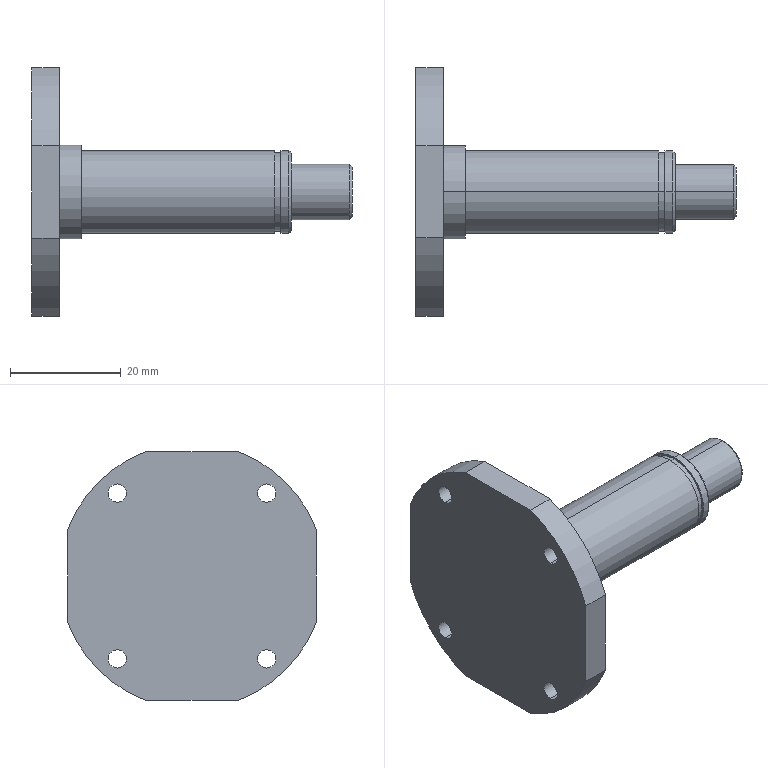Part | SolidWorks | features 3DProfileFeature 1, Chamfer 1, HoleWzd 1, ICE 1, RevCut 1, Revolution 1 | 1 solid | 37 faces | box 58 x 45 x 45 mm | volume 17000 mm3 | cylinder 22 | plane 11 | cone 4 | commonest cylinder face diameters 3.3 x8 15 x4 48 x4 10 x2 14.3 x2 17 x2
STEP:
#1=CARTESIAN_POINT('',(45.1,0.,7.5));
#2=VERTEX_POINT('',#1);
#3=CARTESIAN_POINT('',(45.1,0.,-7.5));
#4=VERTEX_POINT('',#3);
#5=CARTESIAN_POINT('',(45.1,0.,0.));
#6=DIRECTION('',(-1.,0.,0.));
#7=DIRECTION('',(0.,0.,1.));
#8=AXIS2_PLACEMENT_3D('',#5,#6,#7);
#9=CIRCLE('',#8,7.5);
#10=EDGE_CURVE('',#2,#4,#9,.T.);
#11=ORIENTED_EDGE('',*,*,#10,.F.);
#12=CARTESIAN_POINT('',(46.5,0.,7.5));
#13=VERTEX_POINT('',#12);
#14=CARTESIAN_POINT('',(58.,0.,7.5));
#15=DIRECTION('',(1.,0.,0.));
#16=VECTOR('',#15,1000.);
#17=LINE('',#14,#16);
#18=EDGE_CURVE('',#2,#13,#17,.T.);
#19=ORIENTED_EDGE('',*,*,#18,.T.);
#20=CARTESIAN_POINT('',(46.5,0.,-7.5));
#21=VERTEX_POINT('',#20);
#22=CARTESIAN_POINT('',(46.5,0.,0.));
#23=DIRECTION('',(-1.,0.,0.));
#24=DIRECTION('',(0.,0.,-1.));
#25=AXIS2_PLACEMENT_3D('',#22,#23,#24);
#26=CIRCLE('',#25,7.5);
#27=EDGE_CURVE('',#13,#21,#26,.T.);
#28=ORIENTED_EDGE('',*,*,#27,.T.);
#29=CARTESIAN_POINT('',(58.,0.,-7.5));
#30=DIRECTION('',(1.,0.,0.));
#31=VECTOR('',#30,1000.);
#32=LINE('',#29,#31);
#33=EDGE_CURVE('',#4,#21,#32,.T.);
#34=ORIENTED_EDGE('',*,*,#33,.F.);
#35=EDGE_LOOP('',(#11,#19,#28,#34));
#36=FACE_OUTER_BOUND('',#35,.T.);
#37=CARTESIAN_POINT('',(58.,0.,0.));
#38=DIRECTION('',(1.,0.,0.));
#39=DIRECTION('',(0.,0.,-1.));
#40=AXIS2_PLACEMENT_3D('',#37,#38,#39);
#41=CYLINDRICAL_SURFACE('',#40,7.5);
#42=ADVANCED_FACE('',(#36),#41,.T.);
#43=CARTESIAN_POINT('',(47.,0.,-7.));
#44=VERTEX_POINT('',#43);
#45=CARTESIAN_POINT('',(47.,0.,7.));
#46=VERTEX_POINT('',#45);
#47=CARTESIAN_POINT('',(47.,0.,0.));
#48=DIRECTION('',(1.,0.,0.));
#49=DIRECTION('',(0.,0.,-1.));
#50=AXIS2_PLACEMENT_3D('',#47,#48,#49);
#51=CIRCLE('',#50,7.);
#52=EDGE_CURVE('',#44,#46,#51,.T.);
#53=ORIENTED_EDGE('',*,*,#52,.F.);
#54=CARTESIAN_POINT('',(47.,0.,-7.));
#55=DIRECTION('',(-0.7071,0.,-0.7071));
#56=VECTOR('',#55,1000.);
#57=LINE('',#54,#56);
#58=EDGE_CURVE('',#44,#21,#57,.T.);
#59=ORIENTED_EDGE('',*,*,#58,.T.);
#60=ORIENTED_EDGE('',*,*,#27,.F.);
#61=CARTESIAN_POINT('',(47.,0.,7.));
#62=DIRECTION('',(-0.7071,0.,0.7071));
#63=VECTOR('',#62,1000.);
#64=LINE('',#61,#63);
#65=EDGE_CURVE('',#46,#13,#64,.T.);
#66=ORIENTED_EDGE('',*,*,#65,.F.);
#67=EDGE_LOOP('',(#53,#59,#60,#66));
#68=FACE_OUTER_BOUND('',#67,.T.);
#69=CARTESIAN_POINT('',(47.,0.,0.));
#70=DIRECTION('',(-1.,0.,0.));
#71=DIRECTION('',(0.,0.,1.));
#72=AXIS2_PLACEMENT_3D('',#69,#70,#71);
#73=CONICAL_SURFACE('',#72,7.,0.7854);
#74=ADVANCED_FACE('',(#68),#73,.T.);
#75=CARTESIAN_POINT('',(47.,0.,-5.));
#76=VERTEX_POINT('',#75);
#77=CARTESIAN_POINT('',(47.,0.,5.));
#78=VERTEX_POINT('',#77);
#79=CARTESIAN_POINT('',(47.,0.,0.));
#80=DIRECTION('',(1.,0.,0.));
#81=DIRECTION('',(0.,0.,-1.));
#82=AXIS2_PLACEMENT_3D('',#79,#80,#81);
#83=CIRCLE('',#82,5.);
#84=EDGE_CURVE('',#76,#78,#83,.T.);
#85=ORIENTED_EDGE('',*,*,#84,.T.);
#86=CARTESIAN_POINT('',(57.5,0.,5.));
#87=VERTEX_POINT('',#86);
#88=CARTESIAN_POINT('',(58.,0.,5.));
#89=DIRECTION('',(1.,0.,0.));
#90=VECTOR('',#89,1000.);
#91=LINE('',#88,#90);
#92=EDGE_CURVE('',#78,#87,#91,.T.);
#93=ORIENTED_EDGE('',*,*,#92,.T.);
#94=CARTESIAN_POINT('',(57.5,0.,-5.));
#95=VERTEX_POINT('',#94);
#96=CARTESIAN_POINT('',(57.5,0.,0.));
#97=DIRECTION('',(-1.,0.,0.));
#98=DIRECTION('',(0.,0.,-1.));
#99=AXIS2_PLACEMENT_3D('',#96,#97,#98);
#100=CIRCLE('',#99,5.);
#101=EDGE_CURVE('',#87,#95,#100,.T.);
#102=ORIENTED_EDGE('',*,*,#101,.T.);
#103=CARTESIAN_POINT('',(58.,0.,-5.));
#104=DIRECTION('',(1.,0.,0.));
#105=VECTOR('',#104,1000.);
#106=LINE('',#103,#105);
#107=EDGE_CURVE('',#76,#95,#106,.T.);
#108=ORIENTED_EDGE('',*,*,#107,.F.);
#109=EDGE_LOOP('',(#85,#93,#102,#108));
#110=FACE_OUTER_BOUND('',#109,.T.);
#111=CARTESIAN_POINT('',(58.,0.,0.));
#112=DIRECTION('',(1.,0.,0.));
#113=DIRECTION('',(0.,0.,-1.));
#114=AXIS2_PLACEMENT_3D('',#111,#112,#113);
#115=CYLINDRICAL_SURFACE('',#114,5.);
#116=ADVANCED_FACE('',(#110),#115,.T.);
#117=CARTESIAN_POINT('',(58.,0.,-4.5));
#118=VERTEX_POINT('',#117);
#119=CARTESIAN_POINT('',(58.,0.,4.5));
#120=VERTEX_POINT('',#119);
#121=CARTESIAN_POINT('',(58.,0.,0.));
#122=DIRECTION('',(1.,0.,0.));
#123=DIRECTION('',(0.,0.,-1.));
#124=AXIS2_PLACEMENT_3D('',#121,#122,#123);
#125=CIRCLE('',#124,4.5);
#126=EDGE_CURVE('',#118,#120,#125,.T.);
#127=ORIENTED_EDGE('',*,*,#126,.F.);
#128=CARTESIAN_POINT('',(58.,0.,-4.5));
#129=DIRECTION('',(-0.7071,0.,-0.7071));
#130=VECTOR('',#129,1000.);
#131=LINE('',#128,#130);
#132=EDGE_CURVE('',#118,#95,#131,.T.);
#133=ORIENTED_EDGE('',*,*,#132,.T.);
#134=ORIENTED_EDGE('',*,*,#101,.F.);
#135=CARTESIAN_POINT('',(58.,0.,4.5));
#136=DIRECTION('',(-0.7071,0.,0.7071));
#137=VECTOR('',#136,1000.);
#138=LINE('',#135,#137);
#139=EDGE_CURVE('',#120,#87,#138,.T.);
#140=ORIENTED_EDGE('',*,*,#139,.F.);
#141=EDGE_LOOP('',(#127,#133,#134,#140));
#142=FACE_OUTER_BOUND('',#141,.T.);
#143=CARTESIAN_POINT('',(58.,0.,0.));
#144=DIRECTION('',(-1.,0.,0.));
#145=DIRECTION('',(0.,0.,1.));
#146=AXIS2_PLACEMENT_3D('',#143,#144,#145);
#147=CONICAL_SURFACE('',#146,4.5,0.7854);
#148=ADVANCED_FACE('',(#142),#147,.T.);
#149=CARTESIAN_POINT('',(45.1,0.,7.15));
#150=VERTEX_POINT('',#149);
#151=CARTESIAN_POINT('',(45.1,0.,-7.15));
#152=VERTEX_POINT('',#151);
#153=CARTESIAN_POINT('',(45.1,0.,0.));
#154=DIRECTION('',(-1.,0.,0.));
#155=DIRECTION('',(0.,0.,1.));
#156=AXIS2_PLACEMENT_3D('',#153,#154,#155);
#157=CIRCLE('',#156,7.15);
#158=EDGE_CURVE('',#150,#152,#157,.T.);
#159=ORIENTED_EDGE('',*,*,#158,.T.);
#160=CARTESIAN_POINT('',(44.,0.,-7.15));
#161=VERTEX_POINT('',#160);
#162=CARTESIAN_POINT('',(0.,0.,-7.15));
#163=DIRECTION('',(-1.,0.,0.));
#164=VECTOR('',#163,1000.);
#165=LINE('',#162,#164);
#166=EDGE_CURVE('',#152,#161,#165,.T.);
#167=ORIENTED_EDGE('',*,*,#166,.T.);
#168=CARTESIAN_POINT('',(44.,0.,7.15));
#169=VERTEX_POINT('',#168);
#170=CARTESIAN_POINT('',(44.,0.,0.));
#171=DIRECTION('',(-1.,0.,0.));
#172=DIRECTION('',(0.,0.,1.));
#173=AXIS2_PLACEMENT_3D('',#170,#171,#172);
#174=CIRCLE('',#173,7.15);
#175=EDGE_CURVE('',#169,#161,#174,.T.);
#176=ORIENTED_EDGE('',*,*,#175,.F.);
#177=CARTESIAN_POINT('',(0.,0.,7.15));
#178=DIRECTION('',(-1.,0.,0.));
#179=VECTOR('',#178,1000.);
#180=LINE('',#177,#179);
#181=EDGE_CURVE('',#150,#169,#180,.T.);
#182=ORIENTED_EDGE('',*,*,#181,.F.);
#183=EDGE_LOOP('',(#159,#167,#176,#182));
#184=FACE_OUTER_BOUND('',#183,.T.);
#185=CARTESIAN_POINT('',(0.,0.,0.));
#186=DIRECTION('',(-1.,0.,0.));
#187=DIRECTION('',(0.,0.,1.));
#188=AXIS2_PLACEMENT_3D('',#185,#186,#187);
#189=CYLINDRICAL_SURFACE('',#188,7.15);
#190=ADVANCED_FACE('',(#184),#189,.T.);
#191=CARTESIAN_POINT('',(5.,13.5,-13.35));
#192=VERTEX_POINT('',#191);
#193=CARTESIAN_POINT('',(5.,13.5,-16.65));
#194=VERTEX_POINT('',#193);
#195=CARTESIAN_POINT('',(5.,13.5,-15.));
#196=DIRECTION('',(1.,0.,0.));
#197=DIRECTION('',(0.,0.,-1.));
#198=AXIS2_PLACEMENT_3D('',#195,#196,#197);
#199=CIRCLE('',#198,1.65);
#200=EDGE_CURVE('',#192,#194,#199,.T.);
#201=ORIENTED_EDGE('',*,*,#200,.T.);
#202=CARTESIAN_POINT('',(0.,13.5,-16.65));
#203=VERTEX_POINT('',#202);
#204=CARTESIAN_POINT('',(0.,13.5,-16.65));
#205=DIRECTION('',(-1.,0.,0.));
#206=VECTOR('',#205,1000.);
#207=LINE('',#204,#206);
#208=EDGE_CURVE('',#194,#203,#207,.T.);
#209=ORIENTED_EDGE('',*,*,#208,.T.);
#210=CARTESIAN_POINT('',(0.,13.5,-13.35));
#211=VERTEX_POINT('',#210);
#212=CARTESIAN_POINT('',(0.,13.5,-15.));
#213=DIRECTION('',(-1.,0.,0.));
#214=DIRECTION('',(0.,0.,1.));
#215=AXIS2_PLACEMENT_3D('',#212,#213,#214);
#216=CIRCLE('',#215,1.65);
#217=EDGE_CURVE('',#203,#211,#216,.T.);
#218=ORIENTED_EDGE('',*,*,#217,.T.);
#219=CARTESIAN_POINT('',(0.,13.5,-13.35));
#220=DIRECTION('',(-1.,0.,0.));
#221=VECTOR('',#220,1000.);
#222=LINE('',#219,#221);
#223=EDGE_CURVE('',#192,#211,#222,.T.);
#224=ORIENTED_EDGE('',*,*,#223,.F.);
#225=EDGE_LOOP('',(#201,#209,#218,#224));
#226=FACE_OUTER_BOUND('',#225,.T.);
#227=CARTESIAN_POINT('',(0.,13.5,-15.));
#228=DIRECTION('',(-1.,0.,0.));
#229=DIRECTION('',(0.,0.,1.));
#230=AXIS2_PLACEMENT_3D('',#227,#228,#229);
#231=CYLINDRICAL_SURFACE('',#230,1.65);
#232=ADVANCED_FACE('',(#226),#231,.F.);
#233=CARTESIAN_POINT('',(5.,13.5,16.65));
#234=VERTEX_POINT('',#233);
#235=CARTESIAN_POINT('',(5.,13.5,13.35));
#236=VERTEX_POINT('',#235);
#237=CARTESIAN_POINT('',(5.,13.5,15.));
#238=DIRECTION('',(1.,0.,0.));
#239=DIRECTION('',(0.,0.,-1.));
#240=AXIS2_PLACEMENT_3D('',#237,#238,#239);
#241=CIRCLE('',#240,1.65);
#242=EDGE_CURVE('',#234,#236,#241,.T.);
#243=ORIENTED_EDGE('',*,*,#242,.T.);
#244=CARTESIAN_POINT('',(0.,13.5,13.35));
#245=VERTEX_POINT('',#244);
#246=CARTESIAN_POINT('',(0.,13.5,13.35));
#247=DIRECTION('',(-1.,0.,0.));
#248=VECTOR('',#247,1000.);
#249=LINE('',#246,#248);
#250=EDGE_CURVE('',#236,#245,#249,.T.);
#251=ORIENTED_EDGE('',*,*,#250,.T.);
#252=CARTESIAN_POINT('',(0.,13.5,16.65));
#253=VERTEX_POINT('',#252);
#254=CARTESIAN_POINT('',(0.,13.5,15.));
#255=DIRECTION('',(-1.,0.,0.));
#256=DIRECTION('',(0.,0.,1.));
#257=AXIS2_PLACEMENT_3D('',#254,#255,#256);
#258=CIRCLE('',#257,1.65);
#259=EDGE_CURVE('',#245,#253,#258,.T.);
#260=ORIENTED_EDGE('',*,*,#259,.T.);
#261=CARTESIAN_POINT('',(0.,13.5,16.65));
#262=DIRECTION('',(-1.,0.,0.));
#263=VECTOR('',#262,1000.);
#264=LINE('',#261,#263);
#265=EDGE_CURVE('',#234,#253,#264,.T.);
#266=ORIENTED_EDGE('',*,*,#265,.F.);
#267=EDGE_LOOP('',(#243,#251,#260,#266));
#268=FACE_OUTER_BOUND('',#267,.T.);
#269=CARTESIAN_POINT('',(0.,13.5,15.));
#270=DIRECTION('',(-1.,0.,0.));
#271=DIRECTION('',(0.,0.,1.));
#272=AXIS2_PLACEMENT_3D('',#269,#270,#271);
#273=CYLINDRICAL_SURFACE('',#272,1.65);
#274=ADVANCED_FACE('',(#268),#273,.F.);
#275=CARTESIAN_POINT('',(5.,-13.5,-13.35));
#276=VERTEX_POINT('',#275);
#277=CARTESIAN_POINT('',(5.,-13.5,-16.65));
#278=VERTEX_POINT('',#277);
#279=CARTESIAN_POINT('',(5.,-13.5,-15.));
#280=DIRECTION('',(1.,0.,0.));
#281=DIRECTION('',(0.,0.,-1.));
#282=AXIS2_PLACEMENT_3D('',#279,#280,#281);
#283=CIRCLE('',#282,1.65);
#284=EDGE_CURVE('',#276,#278,#283,.T.);
#285=ORIENTED_EDGE('',*,*,#284,.T.);
#286=CARTESIAN_POINT('',(0.,-13.5,-16.65));
#287=VERTEX_POINT('',#286);
#288=CARTESIAN_POINT('',(0.,-13.5,-16.65));
#289=DIRECTION('',(-1.,0.,0.));
#290=VECTOR('',#289,1000.);
#291=LINE('',#288,#290);
#292=EDGE_CURVE('',#278,#287,#291,.T.);
#293=ORIENTED_EDGE('',*,*,#292,.T.);
#294=CARTESIAN_POINT('',(0.,-13.5,-13.35));
#295=VERTEX_POINT('',#294);
#296=CARTESIAN_POINT('',(0.,-13.5,-15.));
#297=DIRECTION('',(-1.,0.,0.));
#298=DIRECTION('',(0.,0.,1.));
#299=AXIS2_PLACEMENT_3D('',#296,#297,#298);
#300=CIRCLE('',#299,1.65);
#301=EDGE_CURVE('',#287,#295,#300,.T.);
#302=ORIENTED_EDGE('',*,*,#301,.T.);
#303=CARTESIAN_POINT('',(0.,-13.5,-13.35));
#304=DIRECTION('',(-1.,0.,0.));
#305=VECTOR('',#304,1000.);
#306=LINE('',#303,#305);
#307=EDGE_CURVE('',#276,#295,#306,.T.);
#308=ORIENTED_EDGE('',*,*,#307,.F.);
#309=EDGE_LOOP('',(#285,#293,#302,#308));
#310=FACE_OUTER_BOUND('',#309,.T.);
#311=CARTESIAN_POINT('',(0.,-13.5,-15.));
#312=DIRECTION('',(-1.,0.,0.));
#313=DIRECTION('',(0.,0.,1.));
#314=AXIS2_PLACEMENT_3D('',#311,#312,#313);
#315=CYLINDRICAL_SURFACE('',#314,1.65);
#316=ADVANCED_FACE('',(#310),#315,.F.);
#317=CARTESIAN_POINT('',(5.,-13.5,16.65));
#318=VERTEX_POINT('',#317);
#319=CARTESIAN_POINT('',(5.,-13.5,13.35));
#320=VERTEX_POINT('',#319);
#321=CARTESIAN_POINT('',(5.,-13.5,15.));
#322=DIRECTION('',(1.,0.,0.));
#323=DIRECTION('',(0.,0.,-1.));
#324=AXIS2_PLACEMENT_3D('',#321,#322,#323);
#325=CIRCLE('',#324,1.65);
#326=EDGE_CURVE('',#318,#320,#325,.T.);
#327=ORIENTED_EDGE('',*,*,#326,.T.);
#328=CARTESIAN_POINT('',(0.,-13.5,13.35));
#329=VERTEX_POINT('',#328);
#330=CARTESIAN_POINT('',(0.,-13.5,13.35));
#331=DIRECTION('',(-1.,0.,0.));
#332=VECTOR('',#331,1000.);
#333=LINE('',#330,#332);
#334=EDGE_CURVE('',#320,#329,#333,.T.);
#335=ORIENTED_EDGE('',*,*,#334,.T.);
#336=CARTESIAN_POINT('',(0.,-13.5,16.65));
#337=VERTEX_POINT('',#336);
#338=CARTESIAN_POINT('',(0.,-13.5,15.));
#339=DIRECTION('',(-1.,0.,0.));
#340=DIRECTION('',(0.,0.,1.));
#341=AXIS2_PLACEMENT_3D('',#338,#339,#340);
#342=CIRCLE('',#341,1.65);
#343=EDGE_CURVE('',#329,#337,#342,.T.);
#344=ORIENTED_EDGE('',*,*,#343,.T.);
#345=CARTESIAN_POINT('',(0.,-13.5,16.65));
#346=DIRECTION('',(-1.,0.,0.));
#347=VECTOR('',#346,1000.);
#348=LINE('',#345,#347);
#349=EDGE_CURVE('',#318,#337,#348,.T.);
#350=ORIENTED_EDGE('',*,*,#349,.F.);
#351=EDGE_LOOP('',(#327,#335,#344,#350));
#352=FACE_OUTER_BOUND('',#351,.T.);
#353=CARTESIAN_POINT('',(0.,-13.5,15.));
#354=DIRECTION('',(-1.,0.,0.));
#355=DIRECTION('',(0.,0.,1.));
#356=AXIS2_PLACEMENT_3D('',#353,#354,#355);
#357=CYLINDRICAL_SURFACE('',#356,1.65);
#358=ADVANCED_FACE('',(#352),#357,.F.);
#359=CARTESIAN_POINT('',(5.,0.,-8.5));
#360=VERTEX_POINT('',#359);
#361=CARTESIAN_POINT('',(5.,0.,8.5));
#362=VERTEX_POINT('',#361);
#363=CARTESIAN_POINT('',(5.,0.,0.));
#364=DIRECTION('',(1.,0.,0.));
#365=DIRECTION('',(0.,0.,-1.));
#366=AXIS2_PLACEMENT_3D('',#363,#364,#365);
#367=CIRCLE('',#366,8.5);
#368=EDGE_CURVE('',#360,#362,#367,.T.);
#369=ORIENTED_EDGE('',*,*,#368,.T.);
#370=CARTESIAN_POINT('',(9.,0.,8.5));
#371=VERTEX_POINT('',#370);
#372=CARTESIAN_POINT('',(58.,0.,8.5));
#373=DIRECTION('',(1.,0.,0.));
#374=VECTOR('',#373,1000.);
#375=LINE('',#372,#374);
#376=EDGE_CURVE('',#362,#371,#375,.T.);
#377=ORIENTED_EDGE('',*,*,#376,.T.);
#378=CARTESIAN_POINT('',(9.,0.,-8.5));
#379=VERTEX_POINT('',#378);
#380=CARTESIAN_POINT('',(9.,0.,0.));
#381=DIRECTION('',(1.,0.,0.));
#382=DIRECTION('',(0.,0.,-1.));
#383=AXIS2_PLACEMENT_3D('',#380,#381,#382);
#384=CIRCLE('',#383,8.5);
#385=EDGE_CURVE('',#379,#371,#384,.T.);
#386=ORIENTED_EDGE('',*,*,#385,.F.);
#387=CARTESIAN_POINT('',(58.,0.,-8.5));
#388=DIRECTION('',(1.,0.,0.));
#389=VECTOR('',#388,1000.);
#390=LINE('',#387,#389);
#391=EDGE_CURVE('',#360,#379,#390,.T.);
#392=ORIENTED_EDGE('',*,*,#391,.F.);
#393=EDGE_LOOP('',(#369,#377,#386,#392));
#394=FACE_OUTER_BOUND('',#393,.T.);
#395=CARTESIAN_POINT('',(58.,0.,0.));
#396=DIRECTION('',(1.,0.,0.));
#397=DIRECTION('',(0.,0.,-1.));
#398=AXIS2_PLACEMENT_3D('',#395,#396,#397);
#399=CYLINDRICAL_SURFACE('',#398,8.5);
#400=ADVANCED_FACE('',(#394),#399,.T.);
#401=CARTESIAN_POINT('',(9.,0.,-7.5));
#402=VERTEX_POINT('',#401);
#403=CARTESIAN_POINT('',(9.,0.,7.5));
#404=VERTEX_POINT('',#403);
#405=CARTESIAN_POINT('',(9.,0.,0.));
#406=DIRECTION('',(1.,0.,0.));
#407=DIRECTION('',(0.,0.,-1.));
#408=AXIS2_PLACEMENT_3D('',#405,#406,#407);
#409=CIRCLE('',#408,7.5);
#410=EDGE_CURVE('',#402,#404,#409,.T.);
#411=ORIENTED_EDGE('',*,*,#410,.T.);
#412=CARTESIAN_POINT('',(44.,0.,7.5));
#413=VERTEX_POINT('',#412);
#414=CARTESIAN_POINT('',(58.,0.,7.5));
#415=DIRECTION('',(1.,0.,0.));
#416=VECTOR('',#415,1000.);
#417=LINE('',#414,#416);
#418=EDGE_CURVE('',#404,#413,#417,.T.);
#419=ORIENTED_EDGE('',*,*,#418,.T.);
#420=CARTESIAN_POINT('',(44.,0.,-7.5));
#421=VERTEX_POINT('',#420);
#422=CARTESIAN_POINT('',(44.,0.,0.));
#423=DIRECTION('',(-1.,0.,0.));
#424=DIRECTION('',(0.,0.,1.));
#425=AXIS2_PLACEMENT_3D('',#422,#423,#424);
#426=CIRCLE('',#425,7.5);
#427=EDGE_CURVE('',#413,#421,#426,.T.);
#428=ORIENTED_EDGE('',*,*,#427,.T.);
#429=CARTESIAN_POINT('',(58.,0.,-7.5));
#430=DIRECTION('',(1.,0.,0.));
#431=VECTOR('',#430,1000.);
#432=LINE('',#429,#431);
#433=EDGE_CURVE('',#402,#421,#432,.T.);
#434=ORIENTED_EDGE('',*,*,#433,.F.);
#435=EDGE_LOOP('',(#411,#419,#428,#434));
#436=FACE_OUTER_BOUND('',#435,.T.);
#437=CARTESIAN_POINT('',(58.,0.,0.));
#438=DIRECTION('',(1.,0.,0.));
#439=DIRECTION('',(0.,0.,-1.));
#440=AXIS2_PLACEMENT_3D('',#437,#438,#439);
#441=CYLINDRICAL_SURFACE('',#440,7.5);
#442=ADVANCED_FACE('',(#436),#441,.T.);
#443=ORIENTED_EDGE('',*,*,#418,.F.);
#444=CARTESIAN_POINT('',(9.,0.,0.));
#445=DIRECTION('',(1.,0.,0.));
#446=DIRECTION('',(0.,0.,-1.));
#447=AXIS2_PLACEMENT_3D('',#444,#445,#446);
#448=CIRCLE('',#447,7.5);
#449=EDGE_CURVE('',#404,#402,#448,.T.);
#450=ORIENTED_EDGE('',*,*,#449,.T.);
#451=ORIENTED_EDGE('',*,*,#433,.T.);
#452=CARTESIAN_POINT('',(44.,0.,0.));
#453=DIRECTION('',(-1.,0.,0.));
#454=DIRECTION('',(0.,0.,1.));
#455=AXIS2_PLACEMENT_3D('',#452,#453,#454);
#456=CIRCLE('',#455,7.5);
#457=EDGE_CURVE('',#421,#413,#456,.T.);
#458=ORIENTED_EDGE('',*,*,#457,.T.);
#459=EDGE_LOOP('',(#443,#450,#451,#458));
#460=FACE_OUTER_BOUND('',#459,.T.);
#461=CARTESIAN_POINT('',(58.,0.,0.));
#462=DIRECTION('',(1.,0.,0.));
#463=DIRECTION('',(0.,0.,-1.));
#464=AXIS2_PLACEMENT_3D('',#461,#462,#463);
#465=CYLINDRICAL_SURFACE('',#464,7.5);
#466=ADVANCED_FACE('',(#460),#465,.T.);
#467=CARTESIAN_POINT('',(0.,13.5,-15.));
#468=DIRECTION('',(-1.,0.,0.));
#469=DIRECTION('',(0.,0.,1.));
#470=AXIS2_PLACEMENT_3D('',#467,#468,#469);
#471=CIRCLE('',#470,1.65);
#472=EDGE_CURVE('',#211,#203,#471,.T.);
#473=ORIENTED_EDGE('',*,*,#472,.F.);
#474=ORIENTED_EDGE('',*,*,#217,.F.);
#475=EDGE_LOOP('',(#473,#474));
#476=FACE_BOUND('',#475,.T.);
#477=CARTESIAN_POINT('',(0.,13.5,15.));
#478=DIRECTION('',(-1.,0.,0.));
#479=DIRECTION('',(0.,0.,1.));
#480=AXIS2_PLACEMENT_3D('',#477,#478,#479);
#481=CIRCLE('',#480,1.65);
#482=EDGE_CURVE('',#253,#245,#481,.T.);
#483=ORIENTED_EDGE('',*,*,#482,.F.);
#484=ORIENTED_EDGE('',*,*,#259,.F.);
#485=EDGE_LOOP('',(#483,#484));
#486=FACE_BOUND('',#485,.T.);
#487=CARTESIAN_POINT('',(0.,-13.5,-15.));
#488=DIRECTION('',(-1.,0.,0.));
#489=DIRECTION('',(0.,0.,1.));
#490=AXIS2_PLACEMENT_3D('',#487,#488,#489);
#491=CIRCLE('',#490,1.65);
#492=EDGE_CURVE('',#295,#287,#491,.T.);
#493=ORIENTED_EDGE('',*,*,#492,.F.);
#494=ORIENTED_EDGE('',*,*,#301,.F.);
#495=EDGE_LOOP('',(#493,#494));
#496=FACE_BOUND('',#495,.T.);
#497=CARTESIAN_POINT('',(0.,-13.5,15.));
#498=DIRECTION('',(-1.,0.,0.));
#499=DIRECTION('',(0.,0.,1.));
#500=AXIS2_PLACEMENT_3D('',#497,#498,#499);
#501=CIRCLE('',#500,1.65);
#502=EDGE_CURVE('',#337,#329,#501,.T.);
#503=ORIENTED_EDGE('',*,*,#502,.F.);
#504=ORIENTED_EDGE('',*,*,#343,.F.);
#505=EDGE_LOOP('',(#503,#504));
#506=FACE_BOUND('',#505,.T.);
#507=CARTESIAN_POINT('',(0.,-8.352,22.5));
#508=VERTEX_POINT('',#507);
#509=CARTESIAN_POINT('',(0.,-22.5,8.352));
#510=VERTEX_POINT('',#509);
#511=CARTESIAN_POINT('',(0.,0.,0.));
#512=DIRECTION('',(1.,0.,0.));
#513=DIRECTION('',(0.,0.,-1.));
#514=AXIS2_PLACEMENT_3D('',#511,#512,#513);
#515=CIRCLE('',#514,24.);
#516=EDGE_CURVE('',#508,#510,#515,.T.);
#517=ORIENTED_EDGE('',*,*,#516,.F.);
#518=CARTESIAN_POINT('',(0.,8.352,22.5));
#519=VERTEX_POINT('',#518);
#520=CARTESIAN_POINT('',(0.,-22.5,22.5));
#521=DIRECTION('',(0.,1.,0.));
#522=VECTOR('',#521,1000.);
#523=LINE('',#520,#522);
#524=EDGE_CURVE('',#508,#519,#523,.T.);
#525=ORIENTED_EDGE('',*,*,#524,.T.);
#526=CARTESIAN_POINT('',(0.,22.5,8.352));
#527=VERTEX_POINT('',#526);
#528=CARTESIAN_POINT('',(0.,0.,0.));
#529=DIRECTION('',(1.,0.,0.));
#530=DIRECTION('',(0.,0.,-1.));
#531=AXIS2_PLACEMENT_3D('',#528,#529,#530);
#532=CIRCLE('',#531,24.);
#533=EDGE_CURVE('',#527,#519,#532,.T.);
#534=ORIENTED_EDGE('',*,*,#533,.F.);
#535=CARTESIAN_POINT('',(0.,22.5,-8.352));
#536=VERTEX_POINT('',#535);
#537=CARTESIAN_POINT('',(0.,22.5,-22.5));
#538=DIRECTION('',(0.,0.,-1.));
#539=VECTOR('',#538,1000.);
#540=LINE('',#537,#539);
#541=EDGE_CURVE('',#527,#536,#540,.T.);
#542=ORIENTED_EDGE('',*,*,#541,.T.);
#543=CARTESIAN_POINT('',(0.,8.352,-22.5));
#544=VERTEX_POINT('',#543);
#545=CARTESIAN_POINT('',(0.,0.,0.));
#546=DIRECTION('',(1.,0.,0.));
#547=DIRECTION('',(0.,0.,-1.));
#548=AXIS2_PLACEMENT_3D('',#545,#546,#547);
#549=CIRCLE('',#548,24.);
#550=EDGE_CURVE('',#544,#536,#549,.T.);
#551=ORIENTED_EDGE('',*,*,#550,.F.);
#552=CARTESIAN_POINT('',(0.,-8.352,-22.5));
#553=VERTEX_POINT('',#552);
#554=CARTESIAN_POINT('',(0.,-22.5,-22.5));
#555=DIRECTION('',(0.,-1.,0.));
#556=VECTOR('',#555,1000.);
#557=LINE('',#554,#556);
#558=EDGE_CURVE('',#544,#553,#557,.T.);
#559=ORIENTED_EDGE('',*,*,#558,.T.);
#560=CARTESIAN_POINT('',(0.,-22.5,-8.352));
#561=VERTEX_POINT('',#560);
#562=CARTESIAN_POINT('',(0.,0.,0.));
#563=DIRECTION('',(1.,0.,0.));
#564=DIRECTION('',(0.,0.,-1.));
#565=AXIS2_PLACEMENT_3D('',#562,#563,#564);
#566=CIRCLE('',#565,24.);
#567=EDGE_CURVE('',#561,#553,#566,.T.);
#568=ORIENTED_EDGE('',*,*,#567,.F.);
#569=CARTESIAN_POINT('',(0.,-22.5,-22.5));
#570=DIRECTION('',(0.,0.,1.));
#571=VECTOR('',#570,1000.);
#572=LINE('',#569,#571);
#573=EDGE_CURVE('',#561,#510,#572,.T.);
#574=ORIENTED_EDGE('',*,*,#573,.T.);
#575=EDGE_LOOP('',(#517,#525,#534,#542,#551,#559,#568,#574));
#576=FACE_OUTER_BOUND('',#575,.T.);
#577=CARTESIAN_POINT('',(0.,0.,0.));
#578=DIRECTION('',(-1.,0.,0.));
#579=DIRECTION('',(0.,0.,1.));
#580=AXIS2_PLACEMENT_3D('',#577,#578,#579);
#581=PLANE('',#580);
#582=ADVANCED_FACE('',(#476,#486,#496,#506,#576),#581,.T.);
#583=CARTESIAN_POINT('',(5.,-8.352,22.5));
#584=VERTEX_POINT('',#583);
#585=CARTESIAN_POINT('',(5.,-22.5,8.352));
#586=VERTEX_POINT('',#585);
#587=CARTESIAN_POINT('',(5.,0.,0.));
#588=DIRECTION('',(1.,0.,0.));
#589=DIRECTION('',(0.,0.,-1.));
#590=AXIS2_PLACEMENT_3D('',#587,#588,#589);
#591=CIRCLE('',#590,24.);
#592=EDGE_CURVE('',#584,#586,#591,.T.);
#593=ORIENTED_EDGE('',*,*,#592,.F.);
#594=CARTESIAN_POINT('',(58.,-8.352,22.5));
#595=DIRECTION('',(-1.,0.,0.));
#596=VECTOR('',#595,1000.);
#597=LINE('',#594,#596);
#598=EDGE_CURVE('',#584,#508,#597,.T.);
#599=ORIENTED_EDGE('',*,*,#598,.T.);
#600=ORIENTED_EDGE('',*,*,#516,.T.);
#601=CARTESIAN_POINT('',(58.,-22.5,8.352));
#602=DIRECTION('',(1.,0.,0.));
#603=VECTOR('',#602,1000.);
#604=LINE('',#601,#603);
#605=EDGE_CURVE('',#510,#586,#604,.T.);
#606=ORIENTED_EDGE('',*,*,#605,.T.);
#607=EDGE_LOOP('',(#593,#599,#600,#606));
#608=FACE_OUTER_BOUND('',#607,.T.);
#609=CARTESIAN_POINT('',(58.,0.,0.));
#610=DIRECTION('',(1.,0.,0.));
#611=DIRECTION('',(0.,0.,-1.));
#612=AXIS2_PLACEMENT_3D('',#609,#610,#611);
#613=CYLINDRICAL_SURFACE('',#612,24.);
#614=ADVANCED_FACE('',(#608),#613,.T.);
#615=ORIENTED_EDGE('',*,*,#533,.T.);
#616=CARTESIAN_POINT('',(5.,8.352,22.5));
#617=VERTEX_POINT('',#616);
#618=CARTESIAN_POINT('',(58.,8.352,22.5));
#619=DIRECTION('',(1.,0.,0.));
#620=VECTOR('',#619,1000.);
#621=LINE('',#618,#620);
#622=EDGE_CURVE('',#519,#617,#621,.T.);
#623=ORIENTED_EDGE('',*,*,#622,.T.);
#624=CARTESIAN_POINT('',(5.,22.5,8.352));
#625=VERTEX_POINT('',#624);
#626=CARTESIAN_POINT('',(5.,0.,0.));
#627=DIRECTION('',(1.,0.,0.));
#628=DIRECTION('',(0.,0.,-1.));
#629=AXIS2_PLACEMENT_3D('',#626,#627,#628);
#630=CIRCLE('',#629,24.);
#631=EDGE_CURVE('',#625,#617,#630,.T.);
#632=ORIENTED_EDGE('',*,*,#631,.F.);
#633=CARTESIAN_POINT('',(58.,22.5,8.352));
#634=DIRECTION('',(-1.,0.,0.));
#635=VECTOR('',#634,1000.);
#636=LINE('',#633,#635);
#637=EDGE_CURVE('',#625,#527,#636,.T.);
#638=ORIENTED_EDGE('',*,*,#637,.T.);
#639=EDGE_LOOP('',(#615,#623,#632,#638));
#640=FACE_OUTER_BOUND('',#639,.T.);
#641=CARTESIAN_POINT('',(58.,0.,0.));
#642=DIRECTION('',(1.,0.,0.));
#643=DIRECTION('',(0.,0.,-1.));
#644=AXIS2_PLACEMENT_3D('',#641,#642,#643);
#645=CYLINDRICAL_SURFACE('',#644,24.);
#646=ADVANCED_FACE('',(#640),#645,.T.);
#647=CARTESIAN_POINT('',(5.,-22.5,-8.352));
#648=VERTEX_POINT('',#647);
#649=CARTESIAN_POINT('',(5.,-8.352,-22.5));
#650=VERTEX_POINT('',#649);
#651=CARTESIAN_POINT('',(5.,0.,0.));
#652=DIRECTION('',(1.,0.,0.));
#653=DIRECTION('',(0.,0.,-1.));
#654=AXIS2_PLACEMENT_3D('',#651,#652,#653);
#655=CIRCLE('',#654,24.);
#656=EDGE_CURVE('',#648,#650,#655,.T.);
#657=ORIENTED_EDGE('',*,*,#656,.F.);
#658=CARTESIAN_POINT('',(58.,-22.5,-8.352));
#659=DIRECTION('',(-1.,0.,0.));
#660=VECTOR('',#659,1000.);
#661=LINE('',#658,#660);
#662=EDGE_CURVE('',#648,#561,#661,.T.);
#663=ORIENTED_EDGE('',*,*,#662,.T.);
#664=ORIENTED_EDGE('',*,*,#567,.T.);
#665=CARTESIAN_POINT('',(58.,-8.352,-22.5));
#666=DIRECTION('',(1.,0.,0.));
#667=VECTOR('',#666,1000.);
#668=LINE('',#665,#667);
#669=EDGE_CURVE('',#553,#650,#668,.T.);
#670=ORIENTED_EDGE('',*,*,#669,.T.);
#671=EDGE_LOOP('',(#657,#663,#664,#670));
#672=FACE_OUTER_BOUND('',#671,.T.);
#673=CARTESIAN_POINT('',(58.,0.,0.));
#674=DIRECTION('',(1.,0.,0.));
#675=DIRECTION('',(0.,0.,-1.));
#676=AXIS2_PLACEMENT_3D('',#673,#674,#675);
#677=CYLINDRICAL_SURFACE('',#676,24.);
#678=ADVANCED_FACE('',(#672),#677,.T.);
#679=CARTESIAN_POINT('',(5.,8.352,-22.5));
#680=VERTEX_POINT('',#679);
#681=CARTESIAN_POINT('',(5.,22.5,-8.352));
#682=VERTEX_POINT('',#681);
#683=CARTESIAN_POINT('',(5.,0.,0.));
#684=DIRECTION('',(1.,0.,0.));
#685=DIRECTION('',(0.,0.,-1.));
#686=AXIS2_PLACEMENT_3D('',#683,#684,#685);
#687=CIRCLE('',#686,24.);
#688=EDGE_CURVE('',#680,#682,#687,.T.);
#689=ORIENTED_EDGE('',*,*,#688,.F.);
#690=CARTESIAN_POINT('',(58.,8.352,-22.5));
#691=DIRECTION('',(-1.,0.,0.));
#692=VECTOR('',#691,1000.);
#693=LINE('',#690,#692);
#694=EDGE_CURVE('',#680,#544,#693,.T.);
#695=ORIENTED_EDGE('',*,*,#694,.T.);
#696=ORIENTED_EDGE('',*,*,#550,.T.);
#697=CARTESIAN_POINT('',(58.,22.5,-8.352));
#698=DIRECTION('',(1.,0.,0.));
#699=VECTOR('',#698,1000.);
#700=LINE('',#697,#699);
#701=EDGE_CURVE('',#536,#682,#700,.T.);
#702=ORIENTED_EDGE('',*,*,#701,.T.);
#703=EDGE_LOOP('',(#689,#695,#696,#702));
#704=FACE_OUTER_BOUND('',#703,.T.);
#705=CARTESIAN_POINT('',(58.,0.,0.));
#706=DIRECTION('',(1.,0.,0.));
#707=DIRECTION('',(0.,0.,-1.));
#708=AXIS2_PLACEMENT_3D('',#705,#706,#707);
#709=CYLINDRICAL_SURFACE('',#708,24.);
#710=ADVANCED_FACE('',(#704),#709,.T.);
#711=ORIENTED_EDGE('',*,*,#200,.F.);
#712=CARTESIAN_POINT('',(5.,13.5,-15.));
#713=DIRECTION('',(1.,0.,0.));
#714=DIRECTION('',(0.,0.,-1.));
#715=AXIS2_PLACEMENT_3D('',#712,#713,#714);
#716=CIRCLE('',#715,1.65);
#717=EDGE_CURVE('',#194,#192,#716,.T.);
#718=ORIENTED_EDGE('',*,*,#717,.F.);
#719=EDGE_LOOP('',(#711,#718));
#720=FACE_BOUND('',#719,.T.);
#721=ORIENTED_EDGE('',*,*,#242,.F.);
#722=CARTESIAN_POINT('',(5.,13.5,15.));
#723=DIRECTION('',(1.,0.,0.));
#724=DIRECTION('',(0.,0.,-1.));
#725=AXIS2_PLACEMENT_3D('',#722,#723,#724);
#726=CIRCLE('',#725,1.65);
#727=EDGE_CURVE('',#236,#234,#726,.T.);
#728=ORIENTED_EDGE('',*,*,#727,.F.);
#729=EDGE_LOOP('',(#721,#728));
#730=FACE_BOUND('',#729,.T.);
#731=ORIENTED_EDGE('',*,*,#284,.F.);
#732=CARTESIAN_POINT('',(5.,-13.5,-15.));
#733=DIRECTION('',(1.,0.,0.));
#734=DIRECTION('',(0.,0.,-1.));
#735=AXIS2_PLACEMENT_3D('',#732,#733,#734);
#736=CIRCLE('',#735,1.65);
#737=EDGE_CURVE('',#278,#276,#736,.T.);
#738=ORIENTED_EDGE('',*,*,#737,.F.);
#739=EDGE_LOOP('',(#731,#738));
#740=FACE_BOUND('',#739,.T.);
#741=ORIENTED_EDGE('',*,*,#326,.F.);
#742=CARTESIAN_POINT('',(5.,-13.5,15.));
#743=DIRECTION('',(1.,0.,0.));
#744=DIRECTION('',(0.,0.,-1.));
#745=AXIS2_PLACEMENT_3D('',#742,#743,#744);
#746=CIRCLE('',#745,1.65);
#747=EDGE_CURVE('',#320,#318,#746,.T.);
#748=ORIENTED_EDGE('',*,*,#747,.F.);
#749=EDGE_LOOP('',(#741,#748));
#750=FACE_BOUND('',#749,.T.);
#751=ORIENTED_EDGE('',*,*,#368,.F.);
#752=CARTESIAN_POINT('',(5.,0.,0.));
#753=DIRECTION('',(1.,0.,0.));
#754=DIRECTION('',(0.,0.,-1.));
#755=AXIS2_PLACEMENT_3D('',#752,#753,#754);
#756=CIRCLE('',#755,8.5);
#757=EDGE_CURVE('',#362,#360,#756,.T.);
#758=ORIENTED_EDGE('',*,*,#757,.F.);
#759=EDGE_LOOP('',(#751,#758));
#760=FACE_BOUND('',#759,.T.);
#761=ORIENTED_EDGE('',*,*,#631,.T.);
#762=CARTESIAN_POINT('',(5.,0.,22.5));
#763=DIRECTION('',(0.,-1.,0.));
#764=VECTOR('',#763,1000.);
#765=LINE('',#762,#764);
#766=EDGE_CURVE('',#617,#584,#765,.T.);
#767=ORIENTED_EDGE('',*,*,#766,.T.);
#768=ORIENTED_EDGE('',*,*,#592,.T.);
#769=CARTESIAN_POINT('',(5.,-22.5,-24.));
#770=DIRECTION('',(0.,0.,-1.));
#771=VECTOR('',#770,1000.);
#772=LINE('',#769,#771);
#773=EDGE_CURVE('',#586,#648,#772,.T.);
#774=ORIENTED_EDGE('',*,*,#773,.T.);
#775=ORIENTED_EDGE('',*,*,#656,.T.);
#776=CARTESIAN_POINT('',(5.,0.,-22.5));
#777=DIRECTION('',(0.,1.,0.));
#778=VECTOR('',#777,1000.);
#779=LINE('',#776,#778);
#780=EDGE_CURVE('',#650,#680,#779,.T.);
#781=ORIENTED_EDGE('',*,*,#780,.T.);
#782=ORIENTED_EDGE('',*,*,#688,.T.);
#783=CARTESIAN_POINT('',(5.,22.5,-24.));
#784=DIRECTION('',(0.,0.,1.));
#785=VECTOR('',#784,1000.);
#786=LINE('',#783,#785);
#787=EDGE_CURVE('',#682,#625,#786,.T.);
#788=ORIENTED_EDGE('',*,*,#787,.T.);
#789=EDGE_LOOP('',(#761,#767,#768,#774,#775,#781,#782,#788));
#790=FACE_OUTER_BOUND('',#789,.T.);
#791=CARTESIAN_POINT('',(5.,0.,-24.));
#792=DIRECTION('',(1.,0.,0.));
#793=DIRECTION('',(0.,0.,-1.));
#794=AXIS2_PLACEMENT_3D('',#791,#792,#793);
#795=PLANE('',#794);
#796=ADVANCED_FACE('',(#720,#730,#740,#750,#760,#790),#795,.T.);
#797=ORIENTED_EDGE('',*,*,#376,.F.);
#798=ORIENTED_EDGE('',*,*,#757,.T.);
#799=ORIENTED_EDGE('',*,*,#391,.T.);
#800=CARTESIAN_POINT('',(9.,0.,0.));
#801=DIRECTION('',(1.,0.,0.));
#802=DIRECTION('',(0.,0.,-1.));
#803=AXIS2_PLACEMENT_3D('',#800,#801,#802);
#804=CIRCLE('',#803,8.5);
#805=EDGE_CURVE('',#371,#379,#804,.T.);
#806=ORIENTED_EDGE('',*,*,#805,.F.);
#807=EDGE_LOOP('',(#797,#798,#799,#806));
#808=FACE_OUTER_BOUND('',#807,.T.);
#809=CARTESIAN_POINT('',(58.,0.,0.));
#810=DIRECTION('',(1.,0.,0.));
#811=DIRECTION('',(0.,0.,-1.));
#812=AXIS2_PLACEMENT_3D('',#809,#810,#811);
#813=CYLINDRICAL_SURFACE('',#812,8.5);
#814=ADVANCED_FACE('',(#808),#813,.T.);
#815=ORIENTED_EDGE('',*,*,#385,.T.);
#816=ORIENTED_EDGE('',*,*,#805,.T.);
#817=EDGE_LOOP('',(#815,#816));
#818=FACE_OUTER_BOUND('',#817,.T.);
#819=ORIENTED_EDGE('',*,*,#410,.F.);
#820=ORIENTED_EDGE('',*,*,#449,.F.);
#821=EDGE_LOOP('',(#819,#820));
#822=FACE_BOUND('',#821,.T.);
#823=CARTESIAN_POINT('',(9.,0.,-8.5));
#824=DIRECTION('',(1.,0.,0.));
#825=DIRECTION('',(0.,0.,-1.));
#826=AXIS2_PLACEMENT_3D('',#823,#824,#825);
#827=PLANE('',#826);
#828=ADVANCED_FACE('',(#818,#822),#827,.T.);
#829=ORIENTED_EDGE('',*,*,#334,.F.);
#830=ORIENTED_EDGE('',*,*,#747,.T.);
#831=ORIENTED_EDGE('',*,*,#349,.T.);
#832=ORIENTED_EDGE('',*,*,#502,.T.);
#833=EDGE_LOOP('',(#829,#830,#831,#832));
#834=FACE_OUTER_BOUND('',#833,.T.);
#835=CARTESIAN_POINT('',(0.,-13.5,15.));
#836=DIRECTION('',(-1.,0.,0.));
#837=DIRECTION('',(0.,0.,1.));
#838=AXIS2_PLACEMENT_3D('',#835,#836,#837);
#839=CYLINDRICAL_SURFACE('',#838,1.65);
#840=ADVANCED_FACE('',(#834),#839,.F.);
#841=ORIENTED_EDGE('',*,*,#292,.F.);
#842=ORIENTED_EDGE('',*,*,#737,.T.);
#843=ORIENTED_EDGE('',*,*,#307,.T.);
#844=ORIENTED_EDGE('',*,*,#492,.T.);
#845=EDGE_LOOP('',(#841,#842,#843,#844));
#846=FACE_OUTER_BOUND('',#845,.T.);
#847=CARTESIAN_POINT('',(0.,-13.5,-15.));
#848=DIRECTION('',(-1.,0.,0.));
#849=DIRECTION('',(0.,0.,1.));
#850=AXIS2_PLACEMENT_3D('',#847,#848,#849);
#851=CYLINDRICAL_SURFACE('',#850,1.65);
#852=ADVANCED_FACE('',(#846),#851,.F.);
#853=ORIENTED_EDGE('',*,*,#250,.F.);
#854=ORIENTED_EDGE('',*,*,#727,.T.);
#855=ORIENTED_EDGE('',*,*,#265,.T.);
#856=ORIENTED_EDGE('',*,*,#482,.T.);
#857=EDGE_LOOP('',(#853,#854,#855,#856));
#858=FACE_OUTER_BOUND('',#857,.T.);
#859=CARTESIAN_POINT('',(0.,13.5,15.));
#860=DIRECTION('',(-1.,0.,0.));
#861=DIRECTION('',(0.,0.,1.));
#862=AXIS2_PLACEMENT_3D('',#859,#860,#861);
#863=CYLINDRICAL_SURFACE('',#862,1.65);
#864=ADVANCED_FACE('',(#858),#863,.F.);
#865=ORIENTED_EDGE('',*,*,#208,.F.);
#866=ORIENTED_EDGE('',*,*,#717,.T.);
#867=ORIENTED_EDGE('',*,*,#223,.T.);
#868=ORIENTED_EDGE('',*,*,#472,.T.);
#869=EDGE_LOOP('',(#865,#866,#867,#868));
#870=FACE_OUTER_BOUND('',#869,.T.);
#871=CARTESIAN_POINT('',(0.,13.5,-15.));
#872=DIRECTION('',(-1.,0.,0.));
#873=DIRECTION('',(0.,0.,1.));
#874=AXIS2_PLACEMENT_3D('',#871,#872,#873);
#875=CYLINDRICAL_SURFACE('',#874,1.65);
#876=ADVANCED_FACE('',(#870),#875,.F.);
#877=ORIENTED_EDGE('',*,*,#787,.F.);
#878=ORIENTED_EDGE('',*,*,#701,.F.);
#879=ORIENTED_EDGE('',*,*,#541,.F.);
#880=ORIENTED_EDGE('',*,*,#637,.F.);
#881=EDGE_LOOP('',(#877,#878,#879,#880));
#882=FACE_OUTER_BOUND('',#881,.T.);
#883=CARTESIAN_POINT('',(10.,22.5,-22.5));
#884=DIRECTION('',(0.,1.,0.));
#885=DIRECTION('',(0.,0.,1.));
#886=AXIS2_PLACEMENT_3D('',#883,#884,#885);
#887=PLANE('',#886);
#888=ADVANCED_FACE('',(#882),#887,.T.);
#889=ORIENTED_EDGE('',*,*,#780,.F.);
#890=ORIENTED_EDGE('',*,*,#669,.F.);
#891=ORIENTED_EDGE('',*,*,#558,.F.);
#892=ORIENTED_EDGE('',*,*,#694,.F.);
#893=EDGE_LOOP('',(#889,#890,#891,#892));
#894=FACE_OUTER_BOUND('',#893,.T.);
#895=CARTESIAN_POINT('',(10.,-22.5,-22.5));
#896=DIRECTION('',(0.,0.,-1.));
#897=DIRECTION('',(-1.,0.,0.));
#898=AXIS2_PLACEMENT_3D('',#895,#896,#897);
#899=PLANE('',#898);
#900=ADVANCED_FACE('',(#894),#899,.T.);
#901=ORIENTED_EDGE('',*,*,#773,.F.);
#902=ORIENTED_EDGE('',*,*,#605,.F.);
#903=ORIENTED_EDGE('',*,*,#573,.F.);
#904=ORIENTED_EDGE('',*,*,#662,.F.);
#905=EDGE_LOOP('',(#901,#902,#903,#904));
#906=FACE_OUTER_BOUND('',#905,.T.);
#907=CARTESIAN_POINT('',(10.,-22.5,-22.5));
#908=DIRECTION('',(0.,-1.,0.));
#909=DIRECTION('',(0.,0.,-1.));
#910=AXIS2_PLACEMENT_3D('',#907,#908,#909);
#911=PLANE('',#910);
#912=ADVANCED_FACE('',(#906),#911,.T.);
#913=ORIENTED_EDGE('',*,*,#766,.F.);
#914=ORIENTED_EDGE('',*,*,#622,.F.);
#915=ORIENTED_EDGE('',*,*,#524,.F.);
#916=ORIENTED_EDGE('',*,*,#598,.F.);
#917=EDGE_LOOP('',(#913,#914,#915,#916));
#918=FACE_OUTER_BOUND('',#917,.T.);
#919=CARTESIAN_POINT('',(10.,-22.5,22.5));
#920=DIRECTION('',(0.,0.,1.));
#921=DIRECTION('',(1.,0.,0.));
#922=AXIS2_PLACEMENT_3D('',#919,#920,#921);
#923=PLANE('',#922);
#924=ADVANCED_FACE('',(#918),#923,.T.);
#925=ORIENTED_EDGE('',*,*,#175,.T.);
#926=CARTESIAN_POINT('',(44.,0.,0.));
#927=DIRECTION('',(-1.,0.,0.));
#928=DIRECTION('',(0.,0.,1.));
#929=AXIS2_PLACEMENT_3D('',#926,#927,#928);
#930=CIRCLE('',#929,7.15);
#931=EDGE_CURVE('',#161,#169,#930,.T.);
#932=ORIENTED_EDGE('',*,*,#931,.T.);
#933=EDGE_LOOP('',(#925,#932));
#934=FACE_BOUND('',#933,.T.);
#935=ORIENTED_EDGE('',*,*,#457,.F.);
#936=ORIENTED_EDGE('',*,*,#427,.F.);
#937=EDGE_LOOP('',(#935,#936));
#938=FACE_OUTER_BOUND('',#937,.T.);
#939=CARTESIAN_POINT('',(44.,0.,-7.5));
#940=DIRECTION('',(1.,0.,0.));
#941=DIRECTION('',(0.,0.,-1.));
#942=AXIS2_PLACEMENT_3D('',#939,#940,#941);
#943=PLANE('',#942);
#944=ADVANCED_FACE('',(#934,#938),#943,.T.);
#945=ORIENTED_EDGE('',*,*,#166,.F.);
#946=CARTESIAN_POINT('',(45.1,0.,0.));
#947=DIRECTION('',(-1.,0.,0.));
#948=DIRECTION('',(0.,0.,1.));
#949=AXIS2_PLACEMENT_3D('',#946,#947,#948);
#950=CIRCLE('',#949,7.15);
#951=EDGE_CURVE('',#152,#150,#950,.T.);
#952=ORIENTED_EDGE('',*,*,#951,.T.);
#953=ORIENTED_EDGE('',*,*,#181,.T.);
#954=ORIENTED_EDGE('',*,*,#931,.F.);
#955=EDGE_LOOP('',(#945,#952,#953,#954));
#956=FACE_OUTER_BOUND('',#955,.T.);
#957=CARTESIAN_POINT('',(0.,0.,0.));
#958=DIRECTION('',(-1.,0.,0.));
#959=DIRECTION('',(0.,0.,1.));
#960=AXIS2_PLACEMENT_3D('',#957,#958,#959);
#961=CYLINDRICAL_SURFACE('',#960,7.15);
#962=ADVANCED_FACE('',(#956),#961,.T.);
#963=CARTESIAN_POINT('',(45.1,0.,0.));
#964=DIRECTION('',(-1.,0.,0.));
#965=DIRECTION('',(0.,0.,1.));
#966=AXIS2_PLACEMENT_3D('',#963,#964,#965);
#967=CIRCLE('',#966,7.5);
#968=EDGE_CURVE('',#4,#2,#967,.T.);
#969=ORIENTED_EDGE('',*,*,#968,.T.);
#970=ORIENTED_EDGE('',*,*,#10,.T.);
#971=EDGE_LOOP('',(#969,#970));
#972=FACE_OUTER_BOUND('',#971,.T.);
#973=ORIENTED_EDGE('',*,*,#158,.F.);
#974=ORIENTED_EDGE('',*,*,#951,.F.);
#975=EDGE_LOOP('',(#973,#974));
#976=FACE_BOUND('',#975,.T.);
#977=CARTESIAN_POINT('',(45.1,0.,-7.5));
#978=DIRECTION('',(-1.,0.,0.));
#979=DIRECTION('',(0.,0.,1.));
#980=AXIS2_PLACEMENT_3D('',#977,#978,#979);
#981=PLANE('',#980);
#982=ADVANCED_FACE('',(#972,#976),#981,.T.);
#983=CARTESIAN_POINT('',(58.,0.,0.));
#984=DIRECTION('',(1.,0.,0.));
#985=DIRECTION('',(0.,0.,-1.));
#986=AXIS2_PLACEMENT_3D('',#983,#984,#985);
#987=CIRCLE('',#986,4.5);
#988=EDGE_CURVE('',#120,#118,#987,.T.);
#989=ORIENTED_EDGE('',*,*,#988,.T.);
#990=ORIENTED_EDGE('',*,*,#126,.T.);
#991=EDGE_LOOP('',(#989,#990));
#992=FACE_OUTER_BOUND('',#991,.T.);
#993=CARTESIAN_POINT('',(58.,0.,-5.));
#994=DIRECTION('',(1.,0.,0.));
#995=DIRECTION('',(0.,0.,-1.));
#996=AXIS2_PLACEMENT_3D('',#993,#994,#995);
#997=PLANE('',#996);
#998=ADVANCED_FACE('',(#992),#997,.T.);
#999=ORIENTED_EDGE('',*,*,#132,.F.);
#1000=ORIENTED_EDGE('',*,*,#988,.F.);
#1001=ORIENTED_EDGE('',*,*,#139,.T.);
#1002=CARTESIAN_POINT('',(57.5,0.,0.));
#1003=DIRECTION('',(-1.,0.,0.));
#1004=DIRECTION('',(0.,0.,-1.));
#1005=AXIS2_PLACEMENT_3D('',#1002,#1003,#1004);
#1006=CIRCLE('',#1005,5.);
#1007=EDGE_CURVE('',#95,#87,#1006,.T.);
#1008=ORIENTED_EDGE('',*,*,#1007,.F.);
#1009=EDGE_LOOP('',(#999,#1000,#1001,#1008));
#1010=FACE_OUTER_BOUND('',#1009,.T.);
#1011=CARTESIAN_POINT('',(58.,0.,0.));
#1012=DIRECTION('',(-1.,0.,0.));
#1013=DIRECTION('',(0.,0.,1.));
#1014=AXIS2_PLACEMENT_3D('',#1011,#1012,#1013);
#1015=CONICAL_SURFACE('',#1014,4.5,0.7854);
#1016=ADVANCED_FACE('',(#1010),#1015,.T.);
#1017=ORIENTED_EDGE('',*,*,#92,.F.);
#1018=CARTESIAN_POINT('',(47.,0.,0.));
#1019=DIRECTION('',(1.,0.,0.));
#1020=DIRECTION('',(0.,0.,-1.));
#1021=AXIS2_PLACEMENT_3D('',#1018,#1019,#1020);
#1022=CIRCLE('',#1021,5.);
#1023=EDGE_CURVE('',#78,#76,#1022,.T.);
#1024=ORIENTED_EDGE('',*,*,#1023,.T.);
#1025=ORIENTED_EDGE('',*,*,#107,.T.);
#1026=ORIENTED_EDGE('',*,*,#1007,.T.);
#1027=EDGE_LOOP('',(#1017,#1024,#1025,#1026));
#1028=FACE_OUTER_BOUND('',#1027,.T.);
#1029=CARTESIAN_POINT('',(58.,0.,0.));
#1030=DIRECTION('',(1.,0.,0.));
#1031=DIRECTION('',(0.,0.,-1.));
#1032=AXIS2_PLACEMENT_3D('',#1029,#1030,#1031);
#1033=CYLINDRICAL_SURFACE('',#1032,5.);
#1034=ADVANCED_FACE('',(#1028),#1033,.T.);
#1035=CARTESIAN_POINT('',(47.,0.,0.));
#1036=DIRECTION('',(1.,0.,0.));
#1037=DIRECTION('',(0.,0.,-1.));
#1038=AXIS2_PLACEMENT_3D('',#1035,#1036,#1037);
#1039=CIRCLE('',#1038,7.);
#1040=EDGE_CURVE('',#46,#44,#1039,.T.);
#1041=ORIENTED_EDGE('',*,*,#1040,.T.);
#1042=ORIENTED_EDGE('',*,*,#52,.T.);
#1043=EDGE_LOOP('',(#1041,#1042));
#1044=FACE_OUTER_BOUND('',#1043,.T.);
#1045=ORIENTED_EDGE('',*,*,#84,.F.);
#1046=ORIENTED_EDGE('',*,*,#1023,.F.);
#1047=EDGE_LOOP('',(#1045,#1046));
#1048=FACE_BOUND('',#1047,.T.);
#1049=CARTESIAN_POINT('',(47.,0.,-7.5));
#1050=DIRECTION('',(1.,0.,0.));
#1051=DIRECTION('',(0.,0.,-1.));
#1052=AXIS2_PLACEMENT_3D('',#1049,#1050,#1051);
#1053=PLANE('',#1052);
#1054=ADVANCED_FACE('',(#1044,#1048),#1053,.T.);
#1055=ORIENTED_EDGE('',*,*,#58,.F.);
#1056=ORIENTED_EDGE('',*,*,#1040,.F.);
#1057=ORIENTED_EDGE('',*,*,#65,.T.);
#1058=CARTESIAN_POINT('',(46.5,0.,0.));
#1059=DIRECTION('',(-1.,0.,0.));
#1060=DIRECTION('',(0.,0.,-1.));
#1061=AXIS2_PLACEMENT_3D('',#1058,#1059,#1060);
#1062=CIRCLE('',#1061,7.5);
#1063=EDGE_CURVE('',#21,#13,#1062,.T.);
#1064=ORIENTED_EDGE('',*,*,#1063,.F.);
#1065=EDGE_LOOP('',(#1055,#1056,#1057,#1064));
#1066=FACE_OUTER_BOUND('',#1065,.T.);
#1067=CARTESIAN_POINT('',(47.,0.,0.));
#1068=DIRECTION('',(-1.,0.,0.));
#1069=DIRECTION('',(0.,0.,1.));
#1070=AXIS2_PLACEMENT_3D('',#1067,#1068,#1069);
#1071=CONICAL_SURFACE('',#1070,7.,0.7854);
#1072=ADVANCED_FACE('',(#1066),#1071,.T.);
#1073=ORIENTED_EDGE('',*,*,#18,.F.);
#1074=ORIENTED_EDGE('',*,*,#968,.F.);
#1075=ORIENTED_EDGE('',*,*,#33,.T.);
#1076=ORIENTED_EDGE('',*,*,#1063,.T.);
#1077=EDGE_LOOP('',(#1073,#1074,#1075,#1076));
#1078=FACE_OUTER_BOUND('',#1077,.T.);
#1079=CARTESIAN_POINT('',(58.,0.,0.));
#1080=DIRECTION('',(1.,0.,0.));
#1081=DIRECTION('',(0.,0.,-1.));
#1082=AXIS2_PLACEMENT_3D('',#1079,#1080,#1081);
#1083=CYLINDRICAL_SURFACE('',#1082,7.5);
#1084=ADVANCED_FACE('',(#1078),#1083,.T.);
#1085=CLOSED_SHELL('',(#42,#74,#116,#148,#190,#232,#274,#316,#358,#400,#442,#466,#582,#614,#646,#678,#710,#796,#814,#828,#840,#852,#864,#876,#888,#900,#912,#924,#944,#962,#982,#998,#1016,#1034,#1054,#1072,#1084));
#1086=MANIFOLD_SOLID_BREP('',#1085);
#1087=CARTESIAN_POINT('',(0.,0.,0.));
#1088=DIRECTION('',(0.,0.,1.));
#1089=DIRECTION('',(1.,0.,0.));
#1090=AXIS2_PLACEMENT_3D('',#1087,#1088,#1089);
#1091=(LENGTH_UNIT()NAMED_UNIT(*)SI_UNIT(.MILLI.,.METRE.));
#1092=UNCERTAINTY_MEASURE_WITH_UNIT(LENGTH_MEASURE(0.00001),#1091,'','');
#1093=(NAMED_UNIT(*)PLANE_ANGLE_UNIT()SI_UNIT($,.RADIAN.));
#1094=(NAMED_UNIT(*)SI_UNIT($,.STERADIAN.)SOLID_ANGLE_UNIT());
#1095=(GEOMETRIC_REPRESENTATION_CONTEXT(3)GLOBAL_UNCERTAINTY_ASSIGNED_CONTEXT((#1092))GLOBAL_UNIT_ASSIGNED_CONTEXT((#1091,#1093,#1094))REPRESENTATION_CONTEXT('',''));
#1096=ADVANCED_BREP_SHAPE_REPRESENTATION('',(#1086,#1090),#1095);